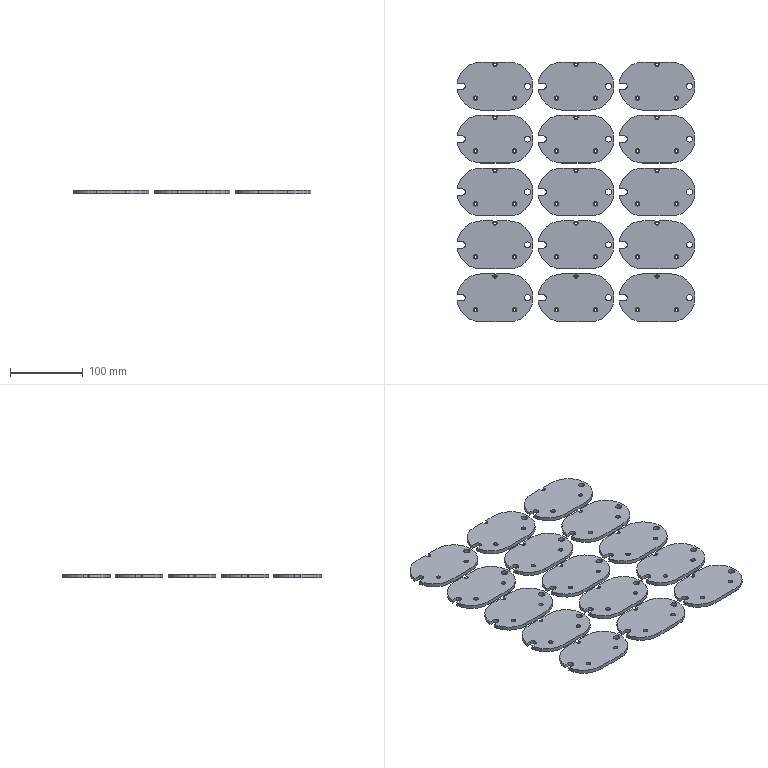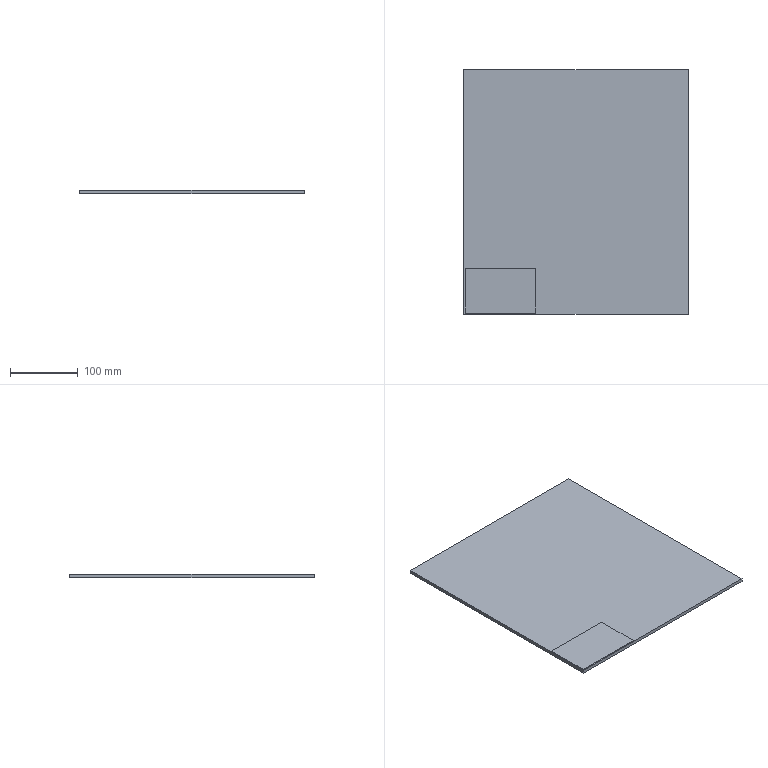CAM job | NX | 3-axis milling, drilling | part box 328.125 x 358 x 5 mm | stock box 332.125 x 362 x 5 mm
Tools:
number,name,description,diameter,corner_radius,flute_length,length,flutes
4,D4,Milling Tool-5 Parameters,4.0,0.0,50.0,75.0,2
6,D6,Milling Tool-5 Parameters,6.0,0.0,50.0,75.0,2
14,D6A45,Milling Tool-5 Parameters,6.0,0.0,50.0,75.0,2
15,5.5ZT,Drilling Tool,3.5,0.0,35.0,50.0,2
13,8.5ZT,Drilling Tool,8.5,0.0,35.0,50.0,2
Operations:
program,operation,operation_type,tool,method,geometry_group,spindle_rpm,surface_speed,feed_per_tooth,feed_cut,feed_plunge,cut_length_mm,path_length_mm,cut_time_min,machine_time_min
1,ZLEVEL_PROFILE,ZLevelMilling,D6,METHOD,A,7500.0,141.0,0.1667,2500.0,1000.0,49653.912,53026.236,20.2,20.538
1,HOLE_MILLING,CylinderMilling,D4,METHOD,A,7500.0,94.0,0.09,1350.0,100.0,2170.621,5723.089,1.608,1.963
1,ZLEVEL_PROFILE_1,ZLevelMilling,D4,METHOD,A,7500.0,94.0,0.1,1500.0,100.0,2060.061,4189.243,1.373,1.586
1,PLANAR_MILL,PlanarMilling,D6A45,METHOD,A,9500.0,179.0,0.0658,1250.0,100.0,5752.783,11585.389,4.602,5.186
1,ZLEVEL_PROFILE_COPY,ZLevelMilling,D6,METHOD,A,7500.0,141.0,0.0667,1000.0,1000.0,4904.978,9026.751,4.905,5.317
2,DRILLING,Operation,D6A45,METHOD,B,5000.0,94.0,0.025,250.0,0.0,16.8,234.869,0.0672,0.089
2,DRILLING_COPY,Operation,5.5ZT,METHOD,B,2000.0,37.0,0.0375,150.0,0.0,22.654,218.864,0.151,0.1707
2,DRILLING_COPY_COPY,Operation,8.5ZT,METHOD,B,2000.0,37.0,0.0375,150.0,0.0,12.054,84.107,0.0804,0.0876
2,PLANAR_MILL_COPY,PlanarMilling,D6A45,METHOD,B,9500.0,179.0,0.0658,1250.0,100.0,364.68,842.936,0.2917,0.3396